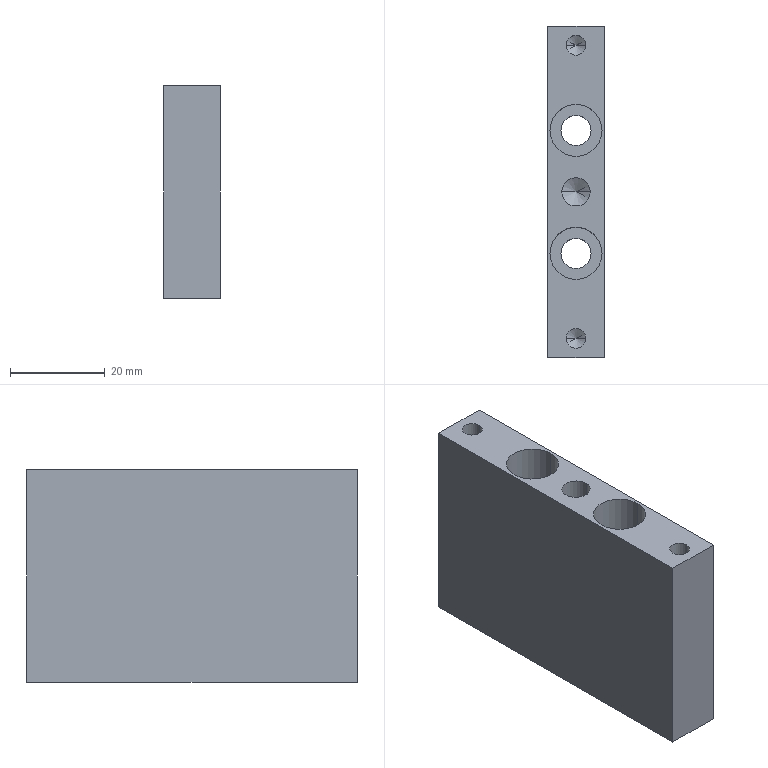Part | SolidWorks | features HoleWzd 5, Extrusion 1, MirrorPattern 1 | 1 solid | 42 faces | box 12 x 70 x 45 mm | volume 30841 mm3 | cylinder 22 | cone 12 | plane 8 | commonest cylinder face diameters 6 x6 2.5 x4 4.2 x4 6.4 x4 11 x4
STEP:
#1=CARTESIAN_POINT('',(3.,-22.5,10.));
#2=VERTEX_POINT('',#1);
#3=CARTESIAN_POINT('',(-3.,-22.5,10.));
#4=VERTEX_POINT('',#3);
#5=CARTESIAN_POINT('',(0.,-22.5,10.));
#6=DIRECTION('',(0.,0.,-1.));
#7=DIRECTION('',(-1.,0.,0.));
#8=AXIS2_PLACEMENT_3D('',#5,#6,#7);
#9=CIRCLE('',#8,3.);
#10=EDGE_CURVE('',#2,#4,#9,.T.);
#11=ORIENTED_EDGE('',*,*,#10,.F.);
#12=CARTESIAN_POINT('',(3.,-22.5,0.));
#13=VERTEX_POINT('',#12);
#14=CARTESIAN_POINT('',(3.,-22.5,0.));
#15=DIRECTION('',(0.,0.,-1.));
#16=VECTOR('',#15,1000.);
#17=LINE('',#14,#16);
#18=EDGE_CURVE('',#2,#13,#17,.T.);
#19=ORIENTED_EDGE('',*,*,#18,.T.);
#20=CARTESIAN_POINT('',(-3.,-22.5,0.));
#21=VERTEX_POINT('',#20);
#22=CARTESIAN_POINT('',(0.,-22.5,0.));
#23=DIRECTION('',(0.,0.,-1.));
#24=DIRECTION('',(-1.,0.,0.));
#25=AXIS2_PLACEMENT_3D('',#22,#23,#24);
#26=CIRCLE('',#25,3.);
#27=EDGE_CURVE('',#13,#21,#26,.T.);
#28=ORIENTED_EDGE('',*,*,#27,.T.);
#29=CARTESIAN_POINT('',(-3.,-22.5,0.));
#30=DIRECTION('',(0.,0.,-1.));
#31=VECTOR('',#30,1000.);
#32=LINE('',#29,#31);
#33=EDGE_CURVE('',#4,#21,#32,.T.);
#34=ORIENTED_EDGE('',*,*,#33,.F.);
#35=EDGE_LOOP('',(#11,#19,#28,#34));
#36=FACE_OUTER_BOUND('',#35,.T.);
#37=CARTESIAN_POINT('',(0.,-22.5,0.));
#38=DIRECTION('',(0.,0.,-1.));
#39=DIRECTION('',(-1.,0.,0.));
#40=AXIS2_PLACEMENT_3D('',#37,#38,#39);
#41=CYLINDRICAL_SURFACE('',#40,3.);
#42=ADVANCED_FACE('',(#36),#41,.F.);
#43=CARTESIAN_POINT('',(0.,-22.5,11.803));
#44=VERTEX_POINT('',#43);
#45=CARTESIAN_POINT('',(-3.,-22.5,10.));
#46=DIRECTION('',(-0.8572,0.,-0.515));
#47=VECTOR('',#46,1000.);
#48=LINE('',#45,#47);
#49=EDGE_CURVE('',#44,#4,#48,.T.);
#50=ORIENTED_EDGE('',*,*,#49,.F.);
#51=CARTESIAN_POINT('',(3.,-22.5,10.));
#52=DIRECTION('',(0.8572,0.,-0.515));
#53=VECTOR('',#52,1000.);
#54=LINE('',#51,#53);
#55=EDGE_CURVE('',#44,#2,#54,.T.);
#56=ORIENTED_EDGE('',*,*,#55,.T.);
#57=ORIENTED_EDGE('',*,*,#10,.T.);
#58=EDGE_LOOP('',(#50,#56,#57));
#59=FACE_OUTER_BOUND('',#58,.T.);
#60=CARTESIAN_POINT('',(0.,-22.5,10.));
#61=DIRECTION('',(0.,0.,-1.));
#62=DIRECTION('',(-1.,0.,0.));
#63=AXIS2_PLACEMENT_3D('',#60,#61,#62);
#64=CONICAL_SURFACE('',#63,3.,1.03);
#65=ADVANCED_FACE('',(#59),#64,.F.);
#66=CARTESIAN_POINT('',(0.,22.5,11.803));
#67=VERTEX_POINT('',#66);
#68=CARTESIAN_POINT('',(-3.,22.5,10.));
#69=VERTEX_POINT('',#68);
#70=CARTESIAN_POINT('',(-3.,22.5,10.));
#71=DIRECTION('',(-0.8572,0.,-0.515));
#72=VECTOR('',#71,1000.);
#73=LINE('',#70,#72);
#74=EDGE_CURVE('',#67,#69,#73,.T.);
#75=ORIENTED_EDGE('',*,*,#74,.F.);
#76=CARTESIAN_POINT('',(3.,22.5,10.));
#77=VERTEX_POINT('',#76);
#78=CARTESIAN_POINT('',(3.,22.5,10.));
#79=DIRECTION('',(0.8572,0.,-0.515));
#80=VECTOR('',#79,1000.);
#81=LINE('',#78,#80);
#82=EDGE_CURVE('',#67,#77,#81,.T.);
#83=ORIENTED_EDGE('',*,*,#82,.T.);
#84=CARTESIAN_POINT('',(0.,22.5,10.));
#85=DIRECTION('',(0.,0.,-1.));
#86=DIRECTION('',(-1.,0.,0.));
#87=AXIS2_PLACEMENT_3D('',#84,#85,#86);
#88=CIRCLE('',#87,3.);
#89=EDGE_CURVE('',#77,#69,#88,.T.);
#90=ORIENTED_EDGE('',*,*,#89,.T.);
#91=EDGE_LOOP('',(#75,#83,#90));
#92=FACE_OUTER_BOUND('',#91,.T.);
#93=CARTESIAN_POINT('',(0.,22.5,10.));
#94=DIRECTION('',(0.,0.,-1.));
#95=DIRECTION('',(-1.,0.,0.));
#96=AXIS2_PLACEMENT_3D('',#93,#94,#95);
#97=CONICAL_SURFACE('',#96,3.,1.03);
#98=ADVANCED_FACE('',(#92),#97,.F.);
#99=ORIENTED_EDGE('',*,*,#89,.F.);
#100=CARTESIAN_POINT('',(3.,22.5,0.));
#101=VERTEX_POINT('',#100);
#102=CARTESIAN_POINT('',(3.,22.5,0.));
#103=DIRECTION('',(0.,0.,-1.));
#104=VECTOR('',#103,1000.);
#105=LINE('',#102,#104);
#106=EDGE_CURVE('',#77,#101,#105,.T.);
#107=ORIENTED_EDGE('',*,*,#106,.T.);
#108=CARTESIAN_POINT('',(-3.,22.5,0.));
#109=VERTEX_POINT('',#108);
#110=CARTESIAN_POINT('',(0.,22.5,0.));
#111=DIRECTION('',(0.,0.,-1.));
#112=DIRECTION('',(-1.,0.,0.));
#113=AXIS2_PLACEMENT_3D('',#110,#111,#112);
#114=CIRCLE('',#113,3.);
#115=EDGE_CURVE('',#101,#109,#114,.T.);
#116=ORIENTED_EDGE('',*,*,#115,.T.);
#117=CARTESIAN_POINT('',(-3.,22.5,0.));
#118=DIRECTION('',(0.,0.,-1.));
#119=VECTOR('',#118,1000.);
#120=LINE('',#117,#119);
#121=EDGE_CURVE('',#69,#109,#120,.T.);
#122=ORIENTED_EDGE('',*,*,#121,.F.);
#123=EDGE_LOOP('',(#99,#107,#116,#122));
#124=FACE_OUTER_BOUND('',#123,.T.);
#125=CARTESIAN_POINT('',(0.,22.5,0.));
#126=DIRECTION('',(0.,0.,-1.));
#127=DIRECTION('',(-1.,0.,0.));
#128=AXIS2_PLACEMENT_3D('',#125,#126,#127);
#129=CYLINDRICAL_SURFACE('',#128,3.);
#130=ADVANCED_FACE('',(#124),#129,.F.);
#131=CARTESIAN_POINT('',(-3.,0.,35.));
#132=VERTEX_POINT('',#131);
#133=CARTESIAN_POINT('',(3.,0.,35.));
#134=VERTEX_POINT('',#133);
#135=CARTESIAN_POINT('',(0.,0.,35.));
#136=DIRECTION('',(0.,0.,1.));
#137=DIRECTION('',(1.,0.,0.));
#138=AXIS2_PLACEMENT_3D('',#135,#136,#137);
#139=CIRCLE('',#138,3.);
#140=EDGE_CURVE('',#132,#134,#139,.T.);
#141=ORIENTED_EDGE('',*,*,#140,.F.);
#142=CARTESIAN_POINT('',(-3.,0.,45.));
#143=VERTEX_POINT('',#142);
#144=CARTESIAN_POINT('',(-3.,0.,45.));
#145=DIRECTION('',(0.,0.,1.));
#146=VECTOR('',#145,1000.);
#147=LINE('',#144,#146);
#148=EDGE_CURVE('',#132,#143,#147,.T.);
#149=ORIENTED_EDGE('',*,*,#148,.T.);
#150=CARTESIAN_POINT('',(3.,0.,45.));
#151=VERTEX_POINT('',#150);
#152=CARTESIAN_POINT('',(0.,0.,45.));
#153=DIRECTION('',(0.,0.,1.));
#154=DIRECTION('',(1.,0.,0.));
#155=AXIS2_PLACEMENT_3D('',#152,#153,#154);
#156=CIRCLE('',#155,3.);
#157=EDGE_CURVE('',#143,#151,#156,.T.);
#158=ORIENTED_EDGE('',*,*,#157,.T.);
#159=CARTESIAN_POINT('',(3.,0.,45.));
#160=DIRECTION('',(0.,0.,1.));
#161=VECTOR('',#160,1000.);
#162=LINE('',#159,#161);
#163=EDGE_CURVE('',#134,#151,#162,.T.);
#164=ORIENTED_EDGE('',*,*,#163,.F.);
#165=EDGE_LOOP('',(#141,#149,#158,#164));
#166=FACE_OUTER_BOUND('',#165,.T.);
#167=CARTESIAN_POINT('',(0.,0.,45.));
#168=DIRECTION('',(0.,0.,1.));
#169=DIRECTION('',(1.,0.,0.));
#170=AXIS2_PLACEMENT_3D('',#167,#168,#169);
#171=CYLINDRICAL_SURFACE('',#170,3.);
#172=ADVANCED_FACE('',(#166),#171,.F.);
#173=CARTESIAN_POINT('',(0.,0.,33.197));
#174=VERTEX_POINT('',#173);
#175=CARTESIAN_POINT('',(3.,0.,35.));
#176=DIRECTION('',(0.8572,0.,0.515));
#177=VECTOR('',#176,1000.);
#178=LINE('',#175,#177);
#179=EDGE_CURVE('',#174,#134,#178,.T.);
#180=ORIENTED_EDGE('',*,*,#179,.F.);
#181=CARTESIAN_POINT('',(-3.,0.,35.));
#182=DIRECTION('',(-0.8572,0.,0.515));
#183=VECTOR('',#182,1000.);
#184=LINE('',#181,#183);
#185=EDGE_CURVE('',#174,#132,#184,.T.);
#186=ORIENTED_EDGE('',*,*,#185,.T.);
#187=ORIENTED_EDGE('',*,*,#140,.T.);
#188=EDGE_LOOP('',(#180,#186,#187));
#189=FACE_OUTER_BOUND('',#188,.T.);
#190=CARTESIAN_POINT('',(0.,0.,35.));
#191=DIRECTION('',(0.,0.,1.));
#192=DIRECTION('',(1.,0.,0.));
#193=AXIS2_PLACEMENT_3D('',#190,#191,#192);
#194=CONICAL_SURFACE('',#193,3.,1.03);
#195=ADVANCED_FACE('',(#189),#194,.F.);
#196=CARTESIAN_POINT('',(-5.5,13.,25.));
#197=VERTEX_POINT('',#196);
#198=CARTESIAN_POINT('',(5.5,13.,25.));
#199=VERTEX_POINT('',#198);
#200=CARTESIAN_POINT('',(0.,13.,25.));
#201=DIRECTION('',(0.,0.,1.));
#202=DIRECTION('',(1.,0.,0.));
#203=AXIS2_PLACEMENT_3D('',#200,#201,#202);
#204=CIRCLE('',#203,5.5);
#205=EDGE_CURVE('',#197,#199,#204,.T.);
#206=ORIENTED_EDGE('',*,*,#205,.F.);
#207=CARTESIAN_POINT('',(-5.5,13.,45.));
#208=VERTEX_POINT('',#207);
#209=CARTESIAN_POINT('',(-5.5,13.,45.));
#210=DIRECTION('',(0.,0.,1.));
#211=VECTOR('',#210,1000.);
#212=LINE('',#209,#211);
#213=EDGE_CURVE('',#197,#208,#212,.T.);
#214=ORIENTED_EDGE('',*,*,#213,.T.);
#215=CARTESIAN_POINT('',(5.5,13.,45.));
#216=VERTEX_POINT('',#215);
#217=CARTESIAN_POINT('',(0.,13.,45.));
#218=DIRECTION('',(0.,0.,1.));
#219=DIRECTION('',(1.,0.,0.));
#220=AXIS2_PLACEMENT_3D('',#217,#218,#219);
#221=CIRCLE('',#220,5.5);
#222=EDGE_CURVE('',#208,#216,#221,.T.);
#223=ORIENTED_EDGE('',*,*,#222,.T.);
#224=CARTESIAN_POINT('',(5.5,13.,45.));
#225=DIRECTION('',(0.,0.,1.));
#226=VECTOR('',#225,1000.);
#227=LINE('',#224,#226);
#228=EDGE_CURVE('',#199,#216,#227,.T.);
#229=ORIENTED_EDGE('',*,*,#228,.F.);
#230=EDGE_LOOP('',(#206,#214,#223,#229));
#231=FACE_OUTER_BOUND('',#230,.T.);
#232=CARTESIAN_POINT('',(0.,13.,45.));
#233=DIRECTION('',(0.,0.,1.));
#234=DIRECTION('',(1.,0.,0.));
#235=AXIS2_PLACEMENT_3D('',#232,#233,#234);
#236=CYLINDRICAL_SURFACE('',#235,5.5);
#237=ADVANCED_FACE('',(#231),#236,.F.);
#238=CARTESIAN_POINT('',(-3.2,13.,0.));
#239=VERTEX_POINT('',#238);
#240=CARTESIAN_POINT('',(3.2,13.,0.));
#241=VERTEX_POINT('',#240);
#242=CARTESIAN_POINT('',(0.,13.,0.));
#243=DIRECTION('',(0.,0.,1.));
#244=DIRECTION('',(1.,0.,0.));
#245=AXIS2_PLACEMENT_3D('',#242,#243,#244);
#246=CIRCLE('',#245,3.2);
#247=EDGE_CURVE('',#239,#241,#246,.T.);
#248=ORIENTED_EDGE('',*,*,#247,.F.);
#249=CARTESIAN_POINT('',(-3.2,13.,25.));
#250=VERTEX_POINT('',#249);
#251=CARTESIAN_POINT('',(-3.2,13.,45.));
#252=DIRECTION('',(0.,0.,1.));
#253=VECTOR('',#252,1000.);
#254=LINE('',#251,#253);
#255=EDGE_CURVE('',#239,#250,#254,.T.);
#256=ORIENTED_EDGE('',*,*,#255,.T.);
#257=CARTESIAN_POINT('',(3.2,13.,25.));
#258=VERTEX_POINT('',#257);
#259=CARTESIAN_POINT('',(0.,13.,25.));
#260=DIRECTION('',(0.,0.,1.));
#261=DIRECTION('',(1.,0.,0.));
#262=AXIS2_PLACEMENT_3D('',#259,#260,#261);
#263=CIRCLE('',#262,3.2);
#264=EDGE_CURVE('',#250,#258,#263,.T.);
#265=ORIENTED_EDGE('',*,*,#264,.T.);
#266=CARTESIAN_POINT('',(3.2,13.,45.));
#267=DIRECTION('',(0.,0.,1.));
#268=VECTOR('',#267,1000.);
#269=LINE('',#266,#268);
#270=EDGE_CURVE('',#241,#258,#269,.T.);
#271=ORIENTED_EDGE('',*,*,#270,.F.);
#272=EDGE_LOOP('',(#248,#256,#265,#271));
#273=FACE_OUTER_BOUND('',#272,.T.);
#274=CARTESIAN_POINT('',(0.,13.,45.));
#275=DIRECTION('',(0.,0.,1.));
#276=DIRECTION('',(1.,0.,0.));
#277=AXIS2_PLACEMENT_3D('',#274,#275,#276);
#278=CYLINDRICAL_SURFACE('',#277,3.2);
#279=ADVANCED_FACE('',(#273),#278,.F.);
#280=CARTESIAN_POINT('',(-5.5,-13.,25.));
#281=VERTEX_POINT('',#280);
#282=CARTESIAN_POINT('',(5.5,-13.,25.));
#283=VERTEX_POINT('',#282);
#284=CARTESIAN_POINT('',(0.,-13.,25.));
#285=DIRECTION('',(0.,0.,1.));
#286=DIRECTION('',(1.,0.,0.));
#287=AXIS2_PLACEMENT_3D('',#284,#285,#286);
#288=CIRCLE('',#287,5.5);
#289=EDGE_CURVE('',#281,#283,#288,.T.);
#290=ORIENTED_EDGE('',*,*,#289,.F.);
#291=CARTESIAN_POINT('',(-5.5,-13.,45.));
#292=VERTEX_POINT('',#291);
#293=CARTESIAN_POINT('',(-5.5,-13.,45.));
#294=DIRECTION('',(0.,0.,1.));
#295=VECTOR('',#294,1000.);
#296=LINE('',#293,#295);
#297=EDGE_CURVE('',#281,#292,#296,.T.);
#298=ORIENTED_EDGE('',*,*,#297,.T.);
#299=CARTESIAN_POINT('',(5.5,-13.,45.));
#300=VERTEX_POINT('',#299);
#301=CARTESIAN_POINT('',(0.,-13.,45.));
#302=DIRECTION('',(0.,0.,1.));
#303=DIRECTION('',(1.,0.,0.));
#304=AXIS2_PLACEMENT_3D('',#301,#302,#303);
#305=CIRCLE('',#304,5.5);
#306=EDGE_CURVE('',#292,#300,#305,.T.);
#307=ORIENTED_EDGE('',*,*,#306,.T.);
#308=CARTESIAN_POINT('',(5.5,-13.,45.));
#309=DIRECTION('',(0.,0.,1.));
#310=VECTOR('',#309,1000.);
#311=LINE('',#308,#310);
#312=EDGE_CURVE('',#283,#300,#311,.T.);
#313=ORIENTED_EDGE('',*,*,#312,.F.);
#314=EDGE_LOOP('',(#290,#298,#307,#313));
#315=FACE_OUTER_BOUND('',#314,.T.);
#316=CARTESIAN_POINT('',(0.,-13.,45.));
#317=DIRECTION('',(0.,0.,1.));
#318=DIRECTION('',(1.,0.,0.));
#319=AXIS2_PLACEMENT_3D('',#316,#317,#318);
#320=CYLINDRICAL_SURFACE('',#319,5.5);
#321=ADVANCED_FACE('',(#315),#320,.F.);
#322=CARTESIAN_POINT('',(-3.2,-13.,0.));
#323=VERTEX_POINT('',#322);
#324=CARTESIAN_POINT('',(3.2,-13.,0.));
#325=VERTEX_POINT('',#324);
#326=CARTESIAN_POINT('',(0.,-13.,0.));
#327=DIRECTION('',(0.,0.,1.));
#328=DIRECTION('',(1.,0.,0.));
#329=AXIS2_PLACEMENT_3D('',#326,#327,#328);
#330=CIRCLE('',#329,3.2);
#331=EDGE_CURVE('',#323,#325,#330,.T.);
#332=ORIENTED_EDGE('',*,*,#331,.F.);
#333=CARTESIAN_POINT('',(-3.2,-13.,25.));
#334=VERTEX_POINT('',#333);
#335=CARTESIAN_POINT('',(-3.2,-13.,45.));
#336=DIRECTION('',(0.,0.,1.));
#337=VECTOR('',#336,1000.);
#338=LINE('',#335,#337);
#339=EDGE_CURVE('',#323,#334,#338,.T.);
#340=ORIENTED_EDGE('',*,*,#339,.T.);
#341=CARTESIAN_POINT('',(3.2,-13.,25.));
#342=VERTEX_POINT('',#341);
#343=CARTESIAN_POINT('',(0.,-13.,25.));
#344=DIRECTION('',(0.,0.,1.));
#345=DIRECTION('',(1.,0.,0.));
#346=AXIS2_PLACEMENT_3D('',#343,#344,#345);
#347=CIRCLE('',#346,3.2);
#348=EDGE_CURVE('',#334,#342,#347,.T.);
#349=ORIENTED_EDGE('',*,*,#348,.T.);
#350=CARTESIAN_POINT('',(3.2,-13.,45.));
#351=DIRECTION('',(0.,0.,1.));
#352=VECTOR('',#351,1000.);
#353=LINE('',#350,#352);
#354=EDGE_CURVE('',#325,#342,#353,.T.);
#355=ORIENTED_EDGE('',*,*,#354,.F.);
#356=EDGE_LOOP('',(#332,#340,#349,#355));
#357=FACE_OUTER_BOUND('',#356,.T.);
#358=CARTESIAN_POINT('',(0.,-13.,45.));
#359=DIRECTION('',(0.,0.,1.));
#360=DIRECTION('',(1.,0.,0.));
#361=AXIS2_PLACEMENT_3D('',#358,#359,#360);
#362=CYLINDRICAL_SURFACE('',#361,3.2);
#363=ADVANCED_FACE('',(#357),#362,.F.);
#364=CARTESIAN_POINT('',(-2.1,31.,26.));
#365=VERTEX_POINT('',#364);
#366=CARTESIAN_POINT('',(2.1,31.,26.));
#367=VERTEX_POINT('',#366);
#368=CARTESIAN_POINT('',(0.,31.,26.));
#369=DIRECTION('',(0.,0.,1.));
#370=DIRECTION('',(1.,0.,0.));
#371=AXIS2_PLACEMENT_3D('',#368,#369,#370);
#372=CIRCLE('',#371,2.1);
#373=EDGE_CURVE('',#365,#367,#372,.T.);
#374=ORIENTED_EDGE('',*,*,#373,.F.);
#375=CARTESIAN_POINT('',(-2.1,31.,45.));
#376=VERTEX_POINT('',#375);
#377=CARTESIAN_POINT('',(-2.1,31.,45.));
#378=DIRECTION('',(0.,0.,1.));
#379=VECTOR('',#378,1000.);
#380=LINE('',#377,#379);
#381=EDGE_CURVE('',#365,#376,#380,.T.);
#382=ORIENTED_EDGE('',*,*,#381,.T.);
#383=CARTESIAN_POINT('',(2.1,31.,45.));
#384=VERTEX_POINT('',#383);
#385=CARTESIAN_POINT('',(0.,31.,45.));
#386=DIRECTION('',(0.,0.,1.));
#387=DIRECTION('',(1.,0.,0.));
#388=AXIS2_PLACEMENT_3D('',#385,#386,#387);
#389=CIRCLE('',#388,2.1);
#390=EDGE_CURVE('',#376,#384,#389,.T.);
#391=ORIENTED_EDGE('',*,*,#390,.T.);
#392=CARTESIAN_POINT('',(2.1,31.,45.));
#393=DIRECTION('',(0.,0.,1.));
#394=VECTOR('',#393,1000.);
#395=LINE('',#392,#394);
#396=EDGE_CURVE('',#367,#384,#395,.T.);
#397=ORIENTED_EDGE('',*,*,#396,.F.);
#398=EDGE_LOOP('',(#374,#382,#391,#397));
#399=FACE_OUTER_BOUND('',#398,.T.);
#400=CARTESIAN_POINT('',(0.,31.,45.));
#401=DIRECTION('',(0.,0.,1.));
#402=DIRECTION('',(1.,0.,0.));
#403=AXIS2_PLACEMENT_3D('',#400,#401,#402);
#404=CYLINDRICAL_SURFACE('',#403,2.1);
#405=ADVANCED_FACE('',(#399),#404,.F.);
#406=CARTESIAN_POINT('',(0.,31.,24.738));
#407=VERTEX_POINT('',#406);
#408=CARTESIAN_POINT('',(2.1,31.,26.));
#409=DIRECTION('',(0.8572,0.,0.515));
#410=VECTOR('',#409,1000.);
#411=LINE('',#408,#410);
#412=EDGE_CURVE('',#407,#367,#411,.T.);
#413=ORIENTED_EDGE('',*,*,#412,.F.);
#414=CARTESIAN_POINT('',(-2.1,31.,26.));
#415=DIRECTION('',(-0.8572,0.,0.515));
#416=VECTOR('',#415,1000.);
#417=LINE('',#414,#416);
#418=EDGE_CURVE('',#407,#365,#417,.T.);
#419=ORIENTED_EDGE('',*,*,#418,.T.);
#420=ORIENTED_EDGE('',*,*,#373,.T.);
#421=EDGE_LOOP('',(#413,#419,#420));
#422=FACE_OUTER_BOUND('',#421,.T.);
#423=CARTESIAN_POINT('',(0.,31.,26.));
#424=DIRECTION('',(0.,0.,1.));
#425=DIRECTION('',(1.,0.,0.));
#426=AXIS2_PLACEMENT_3D('',#423,#424,#425);
#427=CONICAL_SURFACE('',#426,2.1,1.03);
#428=ADVANCED_FACE('',(#422),#427,.F.);
#429=CARTESIAN_POINT('',(-2.1,-31.,26.));
#430=VERTEX_POINT('',#429);
#431=CARTESIAN_POINT('',(2.1,-31.,26.));
#432=VERTEX_POINT('',#431);
#433=CARTESIAN_POINT('',(0.,-31.,26.));
#434=DIRECTION('',(0.,0.,1.));
#435=DIRECTION('',(1.,0.,0.));
#436=AXIS2_PLACEMENT_3D('',#433,#434,#435);
#437=CIRCLE('',#436,2.1);
#438=EDGE_CURVE('',#430,#432,#437,.T.);
#439=ORIENTED_EDGE('',*,*,#438,.F.);
#440=CARTESIAN_POINT('',(-2.1,-31.,45.));
#441=VERTEX_POINT('',#440);
#442=CARTESIAN_POINT('',(-2.1,-31.,45.));
#443=DIRECTION('',(0.,0.,1.));
#444=VECTOR('',#443,1000.);
#445=LINE('',#442,#444);
#446=EDGE_CURVE('',#430,#441,#445,.T.);
#447=ORIENTED_EDGE('',*,*,#446,.T.);
#448=CARTESIAN_POINT('',(2.1,-31.,45.));
#449=VERTEX_POINT('',#448);
#450=CARTESIAN_POINT('',(0.,-31.,45.));
#451=DIRECTION('',(0.,0.,1.));
#452=DIRECTION('',(1.,0.,0.));
#453=AXIS2_PLACEMENT_3D('',#450,#451,#452);
#454=CIRCLE('',#453,2.1);
#455=EDGE_CURVE('',#441,#449,#454,.T.);
#456=ORIENTED_EDGE('',*,*,#455,.T.);
#457=CARTESIAN_POINT('',(2.1,-31.,45.));
#458=DIRECTION('',(0.,0.,1.));
#459=VECTOR('',#458,1000.);
#460=LINE('',#457,#459);
#461=EDGE_CURVE('',#432,#449,#460,.T.);
#462=ORIENTED_EDGE('',*,*,#461,.F.);
#463=EDGE_LOOP('',(#439,#447,#456,#462));
#464=FACE_OUTER_BOUND('',#463,.T.);
#465=CARTESIAN_POINT('',(0.,-31.,45.));
#466=DIRECTION('',(0.,0.,1.));
#467=DIRECTION('',(1.,0.,0.));
#468=AXIS2_PLACEMENT_3D('',#465,#466,#467);
#469=CYLINDRICAL_SURFACE('',#468,2.1);
#470=ADVANCED_FACE('',(#464),#469,.F.);
#471=CARTESIAN_POINT('',(0.,-31.,24.738));
#472=VERTEX_POINT('',#471);
#473=CARTESIAN_POINT('',(2.1,-31.,26.));
#474=DIRECTION('',(0.8572,0.,0.515));
#475=VECTOR('',#474,1000.);
#476=LINE('',#473,#475);
#477=EDGE_CURVE('',#472,#432,#476,.T.);
#478=ORIENTED_EDGE('',*,*,#477,.F.);
#479=CARTESIAN_POINT('',(-2.1,-31.,26.));
#480=DIRECTION('',(-0.8572,0.,0.515));
#481=VECTOR('',#480,1000.);
#482=LINE('',#479,#481);
#483=EDGE_CURVE('',#472,#430,#482,.T.);
#484=ORIENTED_EDGE('',*,*,#483,.T.);
#485=ORIENTED_EDGE('',*,*,#438,.T.);
#486=EDGE_LOOP('',(#478,#484,#485));
#487=FACE_OUTER_BOUND('',#486,.T.);
#488=CARTESIAN_POINT('',(0.,-31.,26.));
#489=DIRECTION('',(0.,0.,1.));
#490=DIRECTION('',(1.,0.,0.));
#491=AXIS2_PLACEMENT_3D('',#488,#489,#490);
#492=CONICAL_SURFACE('',#491,2.1,1.03);
#493=ADVANCED_FACE('',(#487),#492,.F.);
#494=CARTESIAN_POINT('',(-1.25,25.227,10.));
#495=VERTEX_POINT('',#494);
#496=CARTESIAN_POINT('',(0.,25.5,8.75));
#497=VERTEX_POINT('',#496);
#498=CARTESIAN_POINT('',(-1.25,25.227,10.));
#499=CARTESIAN_POINT('',(-1.25,25.227,9.916));
#500=CARTESIAN_POINT('',(-1.242,25.231,9.834));
#501=CARTESIAN_POINT('',(-1.209,25.246,9.673));
#502=CARTESIAN_POINT('',(-1.185,25.256,9.593));
#503=CARTESIAN_POINT('',(-1.09,25.296,9.367));
#504=CARTESIAN_POINT('',(-0.9976,25.332,9.23));
#505=CARTESIAN_POINT('',(-0.7697,25.402,9.002));
#506=CARTESIAN_POINT('',(-0.6318,25.437,8.909));
#507=CARTESIAN_POINT('',(-0.3312,25.486,8.784));
#508=CARTESIAN_POINT('',(-0.1654,25.5,8.75));
#509=CARTESIAN_POINT('',(0.,25.5,8.75));
#510=B_SPLINE_CURVE_WITH_KNOTS('',3,(#498,#499,#500,#501,#502,#503,#504,#505,#506,#507,#508,#509),.UNSPECIFIED.,.F.,.F.,(4,2,2,2,2,4),(0.,0.0002472,0.0004943,0.0009887,0.001483,0.001977),.UNSPECIFIED.);
#511=EDGE_CURVE('',#495,#497,#510,.T.);
#512=ORIENTED_EDGE('',*,*,#511,.T.);
#513=CARTESIAN_POINT('',(0.,35.,8.75));
#514=VERTEX_POINT('',#513);
#515=CARTESIAN_POINT('',(0.,35.,8.75));
#516=DIRECTION('',(0.,1.,0.));
#517=VECTOR('',#516,1000.);
#518=LINE('',#515,#517);
#519=EDGE_CURVE('',#497,#514,#518,.T.);
#520=ORIENTED_EDGE('',*,*,#519,.T.);
#521=CARTESIAN_POINT('',(0.,35.,11.25));
#522=VERTEX_POINT('',#521);
#523=CARTESIAN_POINT('',(0.,35.,10.));
#524=DIRECTION('',(0.,1.,0.));
#525=DIRECTION('',(0.,0.,1.));
#526=AXIS2_PLACEMENT_3D('',#523,#524,#525);
#527=CIRCLE('',#526,1.25);
#528=EDGE_CURVE('',#514,#522,#527,.T.);
#529=ORIENTED_EDGE('',*,*,#528,.T.);
#530=CARTESIAN_POINT('',(0.,23.42,11.25));
#531=VERTEX_POINT('',#530);
#532=CARTESIAN_POINT('',(0.,35.,11.25));
#533=DIRECTION('',(0.,1.,0.));
#534=VECTOR('',#533,1000.);
#535=LINE('',#532,#534);
#536=EDGE_CURVE('',#531,#522,#535,.T.);
#537=ORIENTED_EDGE('',*,*,#536,.F.);
#538=CARTESIAN_POINT('',(0.,23.42,11.25));
#539=CARTESIAN_POINT('',(-0.1196,23.42,11.25));
#540=CARTESIAN_POINT('',(-0.2373,23.423,11.233));
#541=CARTESIAN_POINT('',(-0.4653,23.457,11.166));
#542=CARTESIAN_POINT('',(-0.5713,23.489,11.117));
#543=CARTESIAN_POINT('',(-0.7516,23.596,11.004));
#544=CARTESIAN_POINT('',(-0.8259,23.67,10.942));
#545=CARTESIAN_POINT('',(-0.9473,23.833,10.82));
#546=CARTESIAN_POINT('',(-0.9958,23.923,10.759));
#547=CARTESIAN_POINT('',(-1.118,24.205,10.577));
#548=CARTESIAN_POINT('',(-1.168,24.404,10.461));
#549=CARTESIAN_POINT('',(-1.235,24.811,10.229));
#550=CARTESIAN_POINT('',(-1.25,25.019,10.114));
#551=CARTESIAN_POINT('',(-1.25,25.227,10.));
#552=B_SPLINE_CURVE_WITH_KNOTS('',3,(#538,#539,#540,#541,#542,#543,#544,#545,#546,#547,#548,#549,#550,#551),.UNSPECIFIED.,.F.,.F.,(4,2,2,2,2,2,4),(0.003073,0.003423,0.003774,0.004124,0.004474,0.005175,0.005875),.UNSPECIFIED.);
#553=EDGE_CURVE('',#531,#495,#552,.T.);
#554=ORIENTED_EDGE('',*,*,#553,.T.);
#555=EDGE_LOOP('',(#512,#520,#529,#537,#554));
#556=FACE_OUTER_BOUND('',#555,.T.);
#557=CARTESIAN_POINT('',(0.,35.,10.));
#558=DIRECTION('',(0.,1.,0.));
#559=DIRECTION('',(0.,0.,1.));
#560=AXIS2_PLACEMENT_3D('',#557,#558,#559);
#561=CYLINDRICAL_SURFACE('',#560,1.25);
#562=ADVANCED_FACE('',(#556),#561,.F.);
#563=CARTESIAN_POINT('',(0.,22.5,14.75));
#564=VERTEX_POINT('',#563);
#565=CARTESIAN_POINT('',(0.,22.5,17.25));
#566=VERTEX_POINT('',#565);
#567=CARTESIAN_POINT('',(0.,22.5,16.));
#568=DIRECTION('',(0.,1.,0.));
#569=DIRECTION('',(0.,0.,1.));
#570=AXIS2_PLACEMENT_3D('',#567,#568,#569);
#571=CIRCLE('',#570,1.25);
#572=EDGE_CURVE('',#564,#566,#571,.T.);
#573=ORIENTED_EDGE('',*,*,#572,.F.);
#574=CARTESIAN_POINT('',(0.,35.,14.75));
#575=VERTEX_POINT('',#574);
#576=CARTESIAN_POINT('',(0.,35.,14.75));
#577=DIRECTION('',(0.,1.,0.));
#578=VECTOR('',#577,1000.);
#579=LINE('',#576,#578);
#580=EDGE_CURVE('',#564,#575,#579,.T.);
#581=ORIENTED_EDGE('',*,*,#580,.T.);
#582=CARTESIAN_POINT('',(0.,35.,17.25));
#583=VERTEX_POINT('',#582);
#584=CARTESIAN_POINT('',(0.,35.,16.));
#585=DIRECTION('',(0.,1.,0.));
#586=DIRECTION('',(0.,0.,1.));
#587=AXIS2_PLACEMENT_3D('',#584,#585,#586);
#588=CIRCLE('',#587,1.25);
#589=EDGE_CURVE('',#575,#583,#588,.T.);
#590=ORIENTED_EDGE('',*,*,#589,.T.);
#591=CARTESIAN_POINT('',(0.,35.,17.25));
#592=DIRECTION('',(0.,1.,0.));
#593=VECTOR('',#592,1000.);
#594=LINE('',#591,#593);
#595=EDGE_CURVE('',#566,#583,#594,.T.);
#596=ORIENTED_EDGE('',*,*,#595,.F.);
#597=EDGE_LOOP('',(#573,#581,#590,#596));
#598=FACE_OUTER_BOUND('',#597,.T.);
#599=CARTESIAN_POINT('',(0.,35.,16.));
#600=DIRECTION('',(0.,1.,0.));
#601=DIRECTION('',(0.,0.,1.));
#602=AXIS2_PLACEMENT_3D('',#599,#600,#601);
#603=CYLINDRICAL_SURFACE('',#602,1.25);
#604=ADVANCED_FACE('',(#598),#603,.F.);
#605=CARTESIAN_POINT('',(0.,21.749,16.));
#606=VERTEX_POINT('',#605);
#607=CARTESIAN_POINT('',(0.,22.5,17.25));
#608=DIRECTION('',(0.,0.515,0.8572));
#609=VECTOR('',#608,1000.);
#610=LINE('',#607,#609);
#611=EDGE_CURVE('',#606,#566,#610,.T.);
#612=ORIENTED_EDGE('',*,*,#611,.F.);
#613=CARTESIAN_POINT('',(0.,22.5,14.75));
#614=DIRECTION('',(0.,0.515,-0.8572));
#615=VECTOR('',#614,1000.);
#616=LINE('',#613,#615);
#617=EDGE_CURVE('',#606,#564,#616,.T.);
#618=ORIENTED_EDGE('',*,*,#617,.T.);
#619=ORIENTED_EDGE('',*,*,#572,.T.);
#620=EDGE_LOOP('',(#612,#618,#619));
#621=FACE_OUTER_BOUND('',#620,.T.);
#622=CARTESIAN_POINT('',(0.,22.5,16.));
#623=DIRECTION('',(0.,1.,0.));
#624=DIRECTION('',(0.,0.,1.));
#625=AXIS2_PLACEMENT_3D('',#622,#623,#624);
#626=CONICAL_SURFACE('',#625,1.25,1.03);
#627=ADVANCED_FACE('',(#621),#626,.F.);
#628=CARTESIAN_POINT('',(6.,-35.,0.));
#629=VERTEX_POINT('',#628);
#630=CARTESIAN_POINT('',(6.,35.,0.));
#631=VERTEX_POINT('',#630);
#632=CARTESIAN_POINT('',(6.,35.,0.));
#633=DIRECTION('',(0.,1.,0.));
#634=VECTOR('',#633,1000.);
#635=LINE('',#632,#634);
#636=EDGE_CURVE('',#629,#631,#635,.T.);
#637=ORIENTED_EDGE('',*,*,#636,.T.);
#638=CARTESIAN_POINT('',(6.,35.,45.));
#639=VERTEX_POINT('',#638);
#640=CARTESIAN_POINT('',(6.,35.,45.));
#641=DIRECTION('',(0.,0.,-1.));
#642=VECTOR('',#641,1000.);
#643=LINE('',#640,#642);
#644=EDGE_CURVE('',#639,#631,#643,.T.);
#645=ORIENTED_EDGE('',*,*,#644,.F.);
#646=CARTESIAN_POINT('',(6.,-35.,45.));
#647=VERTEX_POINT('',#646);
#648=CARTESIAN_POINT('',(6.,35.,45.));
#649=DIRECTION('',(0.,1.,0.));
#650=VECTOR('',#649,1000.);
#651=LINE('',#648,#650);
#652=EDGE_CURVE('',#647,#639,#651,.T.);
#653=ORIENTED_EDGE('',*,*,#652,.F.);
#654=CARTESIAN_POINT('',(6.,-35.,45.));
#655=DIRECTION('',(0.,0.,-1.));
#656=VECTOR('',#655,1000.);
#657=LINE('',#654,#656);
#658=EDGE_CURVE('',#647,#629,#657,.T.);
#659=ORIENTED_EDGE('',*,*,#658,.T.);
#660=EDGE_LOOP('',(#637,#645,#653,#659));
#661=FACE_OUTER_BOUND('',#660,.T.);
#662=CARTESIAN_POINT('',(6.,35.,45.));
#663=DIRECTION('',(-1.,0.,0.));
#664=DIRECTION('',(0.,-1.,0.));
#665=AXIS2_PLACEMENT_3D('',#662,#663,#664);
#666=PLANE('',#665);
#667=ADVANCED_FACE('',(#661),#666,.F.);
#668=CARTESIAN_POINT('',(0.,35.,10.));
#669=DIRECTION('',(0.,1.,0.));
#670=DIRECTION('',(0.,0.,1.));
#671=AXIS2_PLACEMENT_3D('',#668,#669,#670);
#672=CIRCLE('',#671,1.25);
#673=EDGE_CURVE('',#522,#514,#672,.T.);
#674=ORIENTED_EDGE('',*,*,#673,.F.);
#675=ORIENTED_EDGE('',*,*,#528,.F.);
#676=EDGE_LOOP('',(#674,#675));
#677=FACE_BOUND('',#676,.T.);
#678=CARTESIAN_POINT('',(0.,35.,16.));
#679=DIRECTION('',(0.,1.,0.));
#680=DIRECTION('',(0.,0.,1.));
#681=AXIS2_PLACEMENT_3D('',#678,#679,#680);
#682=CIRCLE('',#681,1.25);
#683=EDGE_CURVE('',#583,#575,#682,.T.);
#684=ORIENTED_EDGE('',*,*,#683,.F.);
#685=ORIENTED_EDGE('',*,*,#589,.F.);
#686=EDGE_LOOP('',(#684,#685));
#687=FACE_BOUND('',#686,.T.);
#688=CARTESIAN_POINT('',(-6.,35.,0.));
#689=VERTEX_POINT('',#688);
#690=CARTESIAN_POINT('',(-6.,35.,0.));
#691=DIRECTION('',(-1.,0.,0.));
#692=VECTOR('',#691,1000.);
#693=LINE('',#690,#692);
#694=EDGE_CURVE('',#631,#689,#693,.T.);
#695=ORIENTED_EDGE('',*,*,#694,.T.);
#696=CARTESIAN_POINT('',(-6.,35.,45.));
#697=VERTEX_POINT('',#696);
#698=CARTESIAN_POINT('',(-6.,35.,45.));
#699=DIRECTION('',(0.,0.,-1.));
#700=VECTOR('',#699,1000.);
#701=LINE('',#698,#700);
#702=EDGE_CURVE('',#697,#689,#701,.T.);
#703=ORIENTED_EDGE('',*,*,#702,.F.);
#704=CARTESIAN_POINT('',(-6.,35.,45.));
#705=DIRECTION('',(-1.,0.,0.));
#706=VECTOR('',#705,1000.);
#707=LINE('',#704,#706);
#708=EDGE_CURVE('',#639,#697,#707,.T.);
#709=ORIENTED_EDGE('',*,*,#708,.F.);
#710=ORIENTED_EDGE('',*,*,#644,.T.);
#711=EDGE_LOOP('',(#695,#703,#709,#710));
#712=FACE_OUTER_BOUND('',#711,.T.);
#713=CARTESIAN_POINT('',(-6.,35.,45.));
#714=DIRECTION('',(0.,-1.,0.));
#715=DIRECTION('',(0.,0.,-1.));
#716=AXIS2_PLACEMENT_3D('',#713,#714,#715);
#717=PLANE('',#716);
#718=ADVANCED_FACE('',(#677,#687,#712),#717,.F.);
#719=CARTESIAN_POINT('',(-6.,-35.,0.));
#720=VERTEX_POINT('',#719);
#721=CARTESIAN_POINT('',(-6.,35.,0.));
#722=DIRECTION('',(0.,-1.,0.));
#723=VECTOR('',#722,1000.);
#724=LINE('',#721,#723);
#725=EDGE_CURVE('',#689,#720,#724,.T.);
#726=ORIENTED_EDGE('',*,*,#725,.T.);
#727=CARTESIAN_POINT('',(-6.,-35.,45.));
#728=VERTEX_POINT('',#727);
#729=CARTESIAN_POINT('',(-6.,-35.,45.));
#730=DIRECTION('',(0.,0.,-1.));
#731=VECTOR('',#730,1000.);
#732=LINE('',#729,#731);
#733=EDGE_CURVE('',#728,#720,#732,.T.);
#734=ORIENTED_EDGE('',*,*,#733,.F.);
#735=CARTESIAN_POINT('',(-6.,35.,45.));
#736=DIRECTION('',(0.,-1.,0.));
#737=VECTOR('',#736,1000.);
#738=LINE('',#735,#737);
#739=EDGE_CURVE('',#697,#728,#738,.T.);
#740=ORIENTED_EDGE('',*,*,#739,.F.);
#741=ORIENTED_EDGE('',*,*,#702,.T.);
#742=EDGE_LOOP('',(#726,#734,#740,#741));
#743=FACE_OUTER_BOUND('',#742,.T.);
#744=CARTESIAN_POINT('',(-6.,35.,45.));
#745=DIRECTION('',(1.,0.,0.));
#746=DIRECTION('',(0.,1.,0.));
#747=AXIS2_PLACEMENT_3D('',#744,#745,#746);
#748=PLANE('',#747);
#749=ADVANCED_FACE('',(#743),#748,.F.);
#750=CARTESIAN_POINT('',(-6.,-35.,0.));
#751=DIRECTION('',(1.,0.,0.));
#752=VECTOR('',#751,1000.);
#753=LINE('',#750,#752);
#754=EDGE_CURVE('',#720,#629,#753,.T.);
#755=ORIENTED_EDGE('',*,*,#754,.T.);
#756=ORIENTED_EDGE('',*,*,#658,.F.);
#757=CARTESIAN_POINT('',(-6.,-35.,45.));
#758=DIRECTION('',(1.,0.,0.));
#759=VECTOR('',#758,1000.);
#760=LINE('',#757,#759);
#761=EDGE_CURVE('',#728,#647,#760,.T.);
#762=ORIENTED_EDGE('',*,*,#761,.F.);
#763=ORIENTED_EDGE('',*,*,#733,.T.);
#764=EDGE_LOOP('',(#755,#756,#762,#763));
#765=FACE_OUTER_BOUND('',#764,.T.);
#766=CARTESIAN_POINT('',(-6.,-35.,45.));
#767=DIRECTION('',(0.,1.,0.));
#768=DIRECTION('',(0.,0.,1.));
#769=AXIS2_PLACEMENT_3D('',#766,#767,#768);
#770=PLANE('',#769);
#771=ADVANCED_FACE('',(#765),#770,.F.);
#772=CARTESIAN_POINT('',(0.,0.,45.));
#773=DIRECTION('',(0.,0.,1.));
#774=DIRECTION('',(1.,0.,0.));
#775=AXIS2_PLACEMENT_3D('',#772,#773,#774);
#776=CIRCLE('',#775,3.);
#777=EDGE_CURVE('',#151,#143,#776,.T.);
#778=ORIENTED_EDGE('',*,*,#777,.F.);
#779=ORIENTED_EDGE('',*,*,#157,.F.);
#780=EDGE_LOOP('',(#778,#779));
#781=FACE_BOUND('',#780,.T.);
#782=CARTESIAN_POINT('',(0.,13.,45.));
#783=DIRECTION('',(0.,0.,1.));
#784=DIRECTION('',(1.,0.,0.));
#785=AXIS2_PLACEMENT_3D('',#782,#783,#784);
#786=CIRCLE('',#785,5.5);
#787=EDGE_CURVE('',#216,#208,#786,.T.);
#788=ORIENTED_EDGE('',*,*,#787,.F.);
#789=ORIENTED_EDGE('',*,*,#222,.F.);
#790=EDGE_LOOP('',(#788,#789));
#791=FACE_BOUND('',#790,.T.);
#792=CARTESIAN_POINT('',(0.,-13.,45.));
#793=DIRECTION('',(0.,0.,1.));
#794=DIRECTION('',(1.,0.,0.));
#795=AXIS2_PLACEMENT_3D('',#792,#793,#794);
#796=CIRCLE('',#795,5.5);
#797=EDGE_CURVE('',#300,#292,#796,.T.);
#798=ORIENTED_EDGE('',*,*,#797,.F.);
#799=ORIENTED_EDGE('',*,*,#306,.F.);
#800=EDGE_LOOP('',(#798,#799));
#801=FACE_BOUND('',#800,.T.);
#802=CARTESIAN_POINT('',(0.,31.,45.));
#803=DIRECTION('',(0.,0.,1.));
#804=DIRECTION('',(1.,0.,0.));
#805=AXIS2_PLACEMENT_3D('',#802,#803,#804);
#806=CIRCLE('',#805,2.1);
#807=EDGE_CURVE('',#384,#376,#806,.T.);
#808=ORIENTED_EDGE('',*,*,#807,.F.);
#809=ORIENTED_EDGE('',*,*,#390,.F.);
#810=EDGE_LOOP('',(#808,#809));
#811=FACE_BOUND('',#810,.T.);
#812=CARTESIAN_POINT('',(0.,-31.,45.));
#813=DIRECTION('',(0.,0.,1.));
#814=DIRECTION('',(1.,0.,0.));
#815=AXIS2_PLACEMENT_3D('',#812,#813,#814);
#816=CIRCLE('',#815,2.1);
#817=EDGE_CURVE('',#449,#441,#816,.T.);
#818=ORIENTED_EDGE('',*,*,#817,.F.);
#819=ORIENTED_EDGE('',*,*,#455,.F.);
#820=EDGE_LOOP('',(#818,#819));
#821=FACE_BOUND('',#820,.T.);
#822=ORIENTED_EDGE('',*,*,#652,.T.);
#823=ORIENTED_EDGE('',*,*,#708,.T.);
#824=ORIENTED_EDGE('',*,*,#739,.T.);
#825=ORIENTED_EDGE('',*,*,#761,.T.);
#826=EDGE_LOOP('',(#822,#823,#824,#825));
#827=FACE_OUTER_BOUND('',#826,.T.);
#828=CARTESIAN_POINT('',(0.,0.,45.));
#829=DIRECTION('',(0.,0.,1.));
#830=DIRECTION('',(1.,0.,0.));
#831=AXIS2_PLACEMENT_3D('',#828,#829,#830);
#832=PLANE('',#831);
#833=ADVANCED_FACE('',(#781,#791,#801,#811,#821,#827),#832,.T.);
#834=CARTESIAN_POINT('',(0.,-22.5,0.));
#835=DIRECTION('',(0.,0.,-1.));
#836=DIRECTION('',(-1.,0.,0.));
#837=AXIS2_PLACEMENT_3D('',#834,#835,#836);
#838=CIRCLE('',#837,3.);
#839=EDGE_CURVE('',#21,#13,#838,.T.);
#840=ORIENTED_EDGE('',*,*,#839,.F.);
#841=ORIENTED_EDGE('',*,*,#27,.F.);
#842=EDGE_LOOP('',(#840,#841));
#843=FACE_BOUND('',#842,.T.);
#844=CARTESIAN_POINT('',(0.,22.5,0.));
#845=DIRECTION('',(0.,0.,-1.));
#846=DIRECTION('',(-1.,0.,0.));
#847=AXIS2_PLACEMENT_3D('',#844,#845,#846);
#848=CIRCLE('',#847,3.);
#849=EDGE_CURVE('',#109,#101,#848,.T.);
#850=ORIENTED_EDGE('',*,*,#849,.F.);
#851=ORIENTED_EDGE('',*,*,#115,.F.);
#852=EDGE_LOOP('',(#850,#851));
#853=FACE_BOUND('',#852,.T.);
#854=CARTESIAN_POINT('',(0.,13.,0.));
#855=DIRECTION('',(0.,0.,1.));
#856=DIRECTION('',(1.,0.,0.));
#857=AXIS2_PLACEMENT_3D('',#854,#855,#856);
#858=CIRCLE('',#857,3.2);
#859=EDGE_CURVE('',#241,#239,#858,.T.);
#860=ORIENTED_EDGE('',*,*,#859,.T.);
#861=ORIENTED_EDGE('',*,*,#247,.T.);
#862=EDGE_LOOP('',(#860,#861));
#863=FACE_BOUND('',#862,.T.);
#864=CARTESIAN_POINT('',(0.,-13.,0.));
#865=DIRECTION('',(0.,0.,1.));
#866=DIRECTION('',(1.,0.,0.));
#867=AXIS2_PLACEMENT_3D('',#864,#865,#866);
#868=CIRCLE('',#867,3.2);
#869=EDGE_CURVE('',#325,#323,#868,.T.);
#870=ORIENTED_EDGE('',*,*,#869,.T.);
#871=ORIENTED_EDGE('',*,*,#331,.T.);
#872=EDGE_LOOP('',(#870,#871));
#873=FACE_BOUND('',#872,.T.);
#874=ORIENTED_EDGE('',*,*,#636,.F.);
#875=ORIENTED_EDGE('',*,*,#754,.F.);
#876=ORIENTED_EDGE('',*,*,#725,.F.);
#877=ORIENTED_EDGE('',*,*,#694,.F.);
#878=EDGE_LOOP('',(#874,#875,#876,#877));
#879=FACE_OUTER_BOUND('',#878,.T.);
#880=CARTESIAN_POINT('',(0.,0.,0.));
#881=DIRECTION('',(0.,0.,1.));
#882=DIRECTION('',(1.,0.,0.));
#883=AXIS2_PLACEMENT_3D('',#880,#881,#882);
#884=PLANE('',#883);
#885=ADVANCED_FACE('',(#843,#853,#863,#873,#879),#884,.F.);
#886=ORIENTED_EDGE('',*,*,#617,.F.);
#887=ORIENTED_EDGE('',*,*,#611,.T.);
#888=CARTESIAN_POINT('',(0.,22.5,16.));
#889=DIRECTION('',(0.,1.,0.));
#890=DIRECTION('',(0.,0.,1.));
#891=AXIS2_PLACEMENT_3D('',#888,#889,#890);
#892=CIRCLE('',#891,1.25);
#893=EDGE_CURVE('',#566,#564,#892,.T.);
#894=ORIENTED_EDGE('',*,*,#893,.T.);
#895=EDGE_LOOP('',(#886,#887,#894));
#896=FACE_OUTER_BOUND('',#895,.T.);
#897=CARTESIAN_POINT('',(0.,22.5,16.));
#898=DIRECTION('',(0.,1.,0.));
#899=DIRECTION('',(0.,0.,1.));
#900=AXIS2_PLACEMENT_3D('',#897,#898,#899);
#901=CONICAL_SURFACE('',#900,1.25,1.03);
#902=ADVANCED_FACE('',(#896),#901,.F.);
#903=ORIENTED_EDGE('',*,*,#580,.F.);
#904=ORIENTED_EDGE('',*,*,#893,.F.);
#905=ORIENTED_EDGE('',*,*,#595,.T.);
#906=ORIENTED_EDGE('',*,*,#683,.T.);
#907=EDGE_LOOP('',(#903,#904,#905,#906));
#908=FACE_OUTER_BOUND('',#907,.T.);
#909=CARTESIAN_POINT('',(0.,35.,16.));
#910=DIRECTION('',(0.,1.,0.));
#911=DIRECTION('',(0.,0.,1.));
#912=AXIS2_PLACEMENT_3D('',#909,#910,#911);
#913=CYLINDRICAL_SURFACE('',#912,1.25);
#914=ADVANCED_FACE('',(#908),#913,.F.);
#915=ORIENTED_EDGE('',*,*,#519,.F.);
#916=CARTESIAN_POINT('',(1.25,25.227,10.));
#917=VERTEX_POINT('',#916);
#918=CARTESIAN_POINT('',(0.,25.5,8.75));
#919=CARTESIAN_POINT('',(0.08257,25.5,8.75));
#920=CARTESIAN_POINT('',(0.1663,25.496,8.758));
#921=CARTESIAN_POINT('',(0.3273,25.483,8.791));
#922=CARTESIAN_POINT('',(0.4059,25.473,8.815));
#923=CARTESIAN_POINT('',(0.6342,25.436,8.91));
#924=CARTESIAN_POINT('',(0.7704,25.402,9.002));
#925=CARTESIAN_POINT('',(0.9985,25.331,9.231));
#926=CARTESIAN_POINT('',(1.091,25.296,9.368));
#927=CARTESIAN_POINT('',(1.216,25.243,9.668));
#928=CARTESIAN_POINT('',(1.25,25.227,9.833));
#929=CARTESIAN_POINT('',(1.25,25.227,10.));
#930=B_SPLINE_CURVE_WITH_KNOTS('',3,(#918,#919,#920,#921,#922,#923,#924,#925,#926,#927,#928,#929),.UNSPECIFIED.,.F.,.F.,(4,2,2,2,2,4),(0.001977,0.002224,0.002471,0.002964,0.003458,0.003952),.UNSPECIFIED.);
#931=EDGE_CURVE('',#497,#917,#930,.T.);
#932=ORIENTED_EDGE('',*,*,#931,.T.);
#933=CARTESIAN_POINT('',(1.25,25.227,10.));
#934=CARTESIAN_POINT('',(1.25,25.02,10.113));
#935=CARTESIAN_POINT('',(1.235,24.815,10.227));
#936=CARTESIAN_POINT('',(1.17,24.412,10.457));
#937=CARTESIAN_POINT('',(1.12,24.211,10.574));
#938=CARTESIAN_POINT('',(0.998,23.927,10.756));
#939=CARTESIAN_POINT('',(0.9498,23.837,10.817));
#940=CARTESIAN_POINT('',(0.8279,23.672,10.941));
#941=CARTESIAN_POINT('',(0.7545,23.598,11.002));
#942=CARTESIAN_POINT('',(0.5722,23.489,11.117));
#943=CARTESIAN_POINT('',(0.4668,23.457,11.166));
#944=CARTESIAN_POINT('',(0.2386,23.423,11.233));
#945=CARTESIAN_POINT('',(0.1201,23.42,11.25));
#946=CARTESIAN_POINT('',(0.,23.42,11.25));
#947=B_SPLINE_CURVE_WITH_KNOTS('',3,(#933,#934,#935,#936,#937,#938,#939,#940,#941,#942,#943,#944,#945,#946),.UNSPECIFIED.,.F.,.F.,(4,2,2,2,2,2,4),(0.0002596,0.0009629,0.001666,0.002018,0.00237,0.002721,0.003073),.UNSPECIFIED.);
#948=EDGE_CURVE('',#917,#531,#947,.T.);
#949=ORIENTED_EDGE('',*,*,#948,.T.);
#950=ORIENTED_EDGE('',*,*,#536,.T.);
#951=ORIENTED_EDGE('',*,*,#673,.T.);
#952=EDGE_LOOP('',(#915,#932,#949,#950,#951));
#953=FACE_OUTER_BOUND('',#952,.T.);
#954=CARTESIAN_POINT('',(0.,35.,10.));
#955=DIRECTION('',(0.,1.,0.));
#956=DIRECTION('',(0.,0.,1.));
#957=AXIS2_PLACEMENT_3D('',#954,#955,#956);
#958=CYLINDRICAL_SURFACE('',#957,1.25);
#959=ADVANCED_FACE('',(#953),#958,.F.);
#960=ORIENTED_EDGE('',*,*,#483,.F.);
#961=ORIENTED_EDGE('',*,*,#477,.T.);
#962=CARTESIAN_POINT('',(0.,-31.,26.));
#963=DIRECTION('',(0.,0.,1.));
#964=DIRECTION('',(1.,0.,0.));
#965=AXIS2_PLACEMENT_3D('',#962,#963,#964);
#966=CIRCLE('',#965,2.1);
#967=EDGE_CURVE('',#432,#430,#966,.T.);
#968=ORIENTED_EDGE('',*,*,#967,.T.);
#969=EDGE_LOOP('',(#960,#961,#968));
#970=FACE_OUTER_BOUND('',#969,.T.);
#971=CARTESIAN_POINT('',(0.,-31.,26.));
#972=DIRECTION('',(0.,0.,1.));
#973=DIRECTION('',(1.,0.,0.));
#974=AXIS2_PLACEMENT_3D('',#971,#972,#973);
#975=CONICAL_SURFACE('',#974,2.1,1.03);
#976=ADVANCED_FACE('',(#970),#975,.F.);
#977=ORIENTED_EDGE('',*,*,#446,.F.);
#978=ORIENTED_EDGE('',*,*,#967,.F.);
#979=ORIENTED_EDGE('',*,*,#461,.T.);
#980=ORIENTED_EDGE('',*,*,#817,.T.);
#981=EDGE_LOOP('',(#977,#978,#979,#980));
#982=FACE_OUTER_BOUND('',#981,.T.);
#983=CARTESIAN_POINT('',(0.,-31.,45.));
#984=DIRECTION('',(0.,0.,1.));
#985=DIRECTION('',(1.,0.,0.));
#986=AXIS2_PLACEMENT_3D('',#983,#984,#985);
#987=CYLINDRICAL_SURFACE('',#986,2.1);
#988=ADVANCED_FACE('',(#982),#987,.F.);
#989=ORIENTED_EDGE('',*,*,#418,.F.);
#990=ORIENTED_EDGE('',*,*,#412,.T.);
#991=CARTESIAN_POINT('',(0.,31.,26.));
#992=DIRECTION('',(0.,0.,1.));
#993=DIRECTION('',(1.,0.,0.));
#994=AXIS2_PLACEMENT_3D('',#991,#992,#993);
#995=CIRCLE('',#994,2.1);
#996=EDGE_CURVE('',#367,#365,#995,.T.);
#997=ORIENTED_EDGE('',*,*,#996,.T.);
#998=EDGE_LOOP('',(#989,#990,#997));
#999=FACE_OUTER_BOUND('',#998,.T.);
#1000=CARTESIAN_POINT('',(0.,31.,26.));
#1001=DIRECTION('',(0.,0.,1.));
#1002=DIRECTION('',(1.,0.,0.));
#1003=AXIS2_PLACEMENT_3D('',#1000,#1001,#1002);
#1004=CONICAL_SURFACE('',#1003,2.1,1.03);
#1005=ADVANCED_FACE('',(#999),#1004,.F.);
#1006=ORIENTED_EDGE('',*,*,#381,.F.);
#1007=ORIENTED_EDGE('',*,*,#996,.F.);
#1008=ORIENTED_EDGE('',*,*,#396,.T.);
#1009=ORIENTED_EDGE('',*,*,#807,.T.);
#1010=EDGE_LOOP('',(#1006,#1007,#1008,#1009));
#1011=FACE_OUTER_BOUND('',#1010,.T.);
#1012=CARTESIAN_POINT('',(0.,31.,45.));
#1013=DIRECTION('',(0.,0.,1.));
#1014=DIRECTION('',(1.,0.,0.));
#1015=AXIS2_PLACEMENT_3D('',#1012,#1013,#1014);
#1016=CYLINDRICAL_SURFACE('',#1015,2.1);
#1017=ADVANCED_FACE('',(#1011),#1016,.F.);
#1018=ORIENTED_EDGE('',*,*,#339,.F.);
#1019=ORIENTED_EDGE('',*,*,#869,.F.);
#1020=ORIENTED_EDGE('',*,*,#354,.T.);
#1021=CARTESIAN_POINT('',(0.,-13.,25.));
#1022=DIRECTION('',(0.,0.,1.));
#1023=DIRECTION('',(1.,0.,0.));
#1024=AXIS2_PLACEMENT_3D('',#1021,#1022,#1023);
#1025=CIRCLE('',#1024,3.2);
#1026=EDGE_CURVE('',#342,#334,#1025,.T.);
#1027=ORIENTED_EDGE('',*,*,#1026,.T.);
#1028=EDGE_LOOP('',(#1018,#1019,#1020,#1027));
#1029=FACE_OUTER_BOUND('',#1028,.T.);
#1030=CARTESIAN_POINT('',(0.,-13.,45.));
#1031=DIRECTION('',(0.,0.,1.));
#1032=DIRECTION('',(1.,0.,0.));
#1033=AXIS2_PLACEMENT_3D('',#1030,#1031,#1032);
#1034=CYLINDRICAL_SURFACE('',#1033,3.2);
#1035=ADVANCED_FACE('',(#1029),#1034,.F.);
#1036=ORIENTED_EDGE('',*,*,#1026,.F.);
#1037=ORIENTED_EDGE('',*,*,#348,.F.);
#1038=EDGE_LOOP('',(#1036,#1037));
#1039=FACE_BOUND('',#1038,.T.);
#1040=CARTESIAN_POINT('',(0.,-13.,25.));
#1041=DIRECTION('',(0.,0.,1.));
#1042=DIRECTION('',(1.,0.,0.));
#1043=AXIS2_PLACEMENT_3D('',#1040,#1041,#1042);
#1044=CIRCLE('',#1043,5.5);
#1045=EDGE_CURVE('',#283,#281,#1044,.T.);
#1046=ORIENTED_EDGE('',*,*,#1045,.T.);
#1047=ORIENTED_EDGE('',*,*,#289,.T.);
#1048=EDGE_LOOP('',(#1046,#1047));
#1049=FACE_OUTER_BOUND('',#1048,.T.);
#1050=CARTESIAN_POINT('',(3.2,-13.,25.));
#1051=DIRECTION('',(0.,0.,-1.));
#1052=DIRECTION('',(-1.,0.,0.));
#1053=AXIS2_PLACEMENT_3D('',#1050,#1051,#1052);
#1054=PLANE('',#1053);
#1055=ADVANCED_FACE('',(#1039,#1049),#1054,.F.);
#1056=ORIENTED_EDGE('',*,*,#297,.F.);
#1057=ORIENTED_EDGE('',*,*,#1045,.F.);
#1058=ORIENTED_EDGE('',*,*,#312,.T.);
#1059=ORIENTED_EDGE('',*,*,#797,.T.);
#1060=EDGE_LOOP('',(#1056,#1057,#1058,#1059));
#1061=FACE_OUTER_BOUND('',#1060,.T.);
#1062=CARTESIAN_POINT('',(0.,-13.,45.));
#1063=DIRECTION('',(0.,0.,1.));
#1064=DIRECTION('',(1.,0.,0.));
#1065=AXIS2_PLACEMENT_3D('',#1062,#1063,#1064);
#1066=CYLINDRICAL_SURFACE('',#1065,5.5);
#1067=ADVANCED_FACE('',(#1061),#1066,.F.);
#1068=ORIENTED_EDGE('',*,*,#255,.F.);
#1069=ORIENTED_EDGE('',*,*,#859,.F.);
#1070=ORIENTED_EDGE('',*,*,#270,.T.);
#1071=CARTESIAN_POINT('',(0.,13.,25.));
#1072=DIRECTION('',(0.,0.,1.));
#1073=DIRECTION('',(1.,0.,0.));
#1074=AXIS2_PLACEMENT_3D('',#1071,#1072,#1073);
#1075=CIRCLE('',#1074,3.2);
#1076=EDGE_CURVE('',#258,#250,#1075,.T.);
#1077=ORIENTED_EDGE('',*,*,#1076,.T.);
#1078=EDGE_LOOP('',(#1068,#1069,#1070,#1077));
#1079=FACE_OUTER_BOUND('',#1078,.T.);
#1080=CARTESIAN_POINT('',(0.,13.,45.));
#1081=DIRECTION('',(0.,0.,1.));
#1082=DIRECTION('',(1.,0.,0.));
#1083=AXIS2_PLACEMENT_3D('',#1080,#1081,#1082);
#1084=CYLINDRICAL_SURFACE('',#1083,3.2);
#1085=ADVANCED_FACE('',(#1079),#1084,.F.);
#1086=ORIENTED_EDGE('',*,*,#1076,.F.);
#1087=ORIENTED_EDGE('',*,*,#264,.F.);
#1088=EDGE_LOOP('',(#1086,#1087));
#1089=FACE_BOUND('',#1088,.T.);
#1090=CARTESIAN_POINT('',(0.,13.,25.));
#1091=DIRECTION('',(0.,0.,1.));
#1092=DIRECTION('',(1.,0.,0.));
#1093=AXIS2_PLACEMENT_3D('',#1090,#1091,#1092);
#1094=CIRCLE('',#1093,5.5);
#1095=EDGE_CURVE('',#199,#197,#1094,.T.);
#1096=ORIENTED_EDGE('',*,*,#1095,.T.);
#1097=ORIENTED_EDGE('',*,*,#205,.T.);
#1098=EDGE_LOOP('',(#1096,#1097));
#1099=FACE_OUTER_BOUND('',#1098,.T.);
#1100=CARTESIAN_POINT('',(3.2,13.,25.));
#1101=DIRECTION('',(0.,0.,-1.));
#1102=DIRECTION('',(-1.,0.,0.));
#1103=AXIS2_PLACEMENT_3D('',#1100,#1101,#1102);
#1104=PLANE('',#1103);
#1105=ADVANCED_FACE('',(#1089,#1099),#1104,.F.);
#1106=ORIENTED_EDGE('',*,*,#213,.F.);
#1107=ORIENTED_EDGE('',*,*,#1095,.F.);
#1108=ORIENTED_EDGE('',*,*,#228,.T.);
#1109=ORIENTED_EDGE('',*,*,#787,.T.);
#1110=EDGE_LOOP('',(#1106,#1107,#1108,#1109));
#1111=FACE_OUTER_BOUND('',#1110,.T.);
#1112=CARTESIAN_POINT('',(0.,13.,45.));
#1113=DIRECTION('',(0.,0.,1.));
#1114=DIRECTION('',(1.,0.,0.));
#1115=AXIS2_PLACEMENT_3D('',#1112,#1113,#1114);
#1116=CYLINDRICAL_SURFACE('',#1115,5.5);
#1117=ADVANCED_FACE('',(#1111),#1116,.F.);
#1118=ORIENTED_EDGE('',*,*,#185,.F.);
#1119=ORIENTED_EDGE('',*,*,#179,.T.);
#1120=CARTESIAN_POINT('',(0.,0.,35.));
#1121=DIRECTION('',(0.,0.,1.));
#1122=DIRECTION('',(1.,0.,0.));
#1123=AXIS2_PLACEMENT_3D('',#1120,#1121,#1122);
#1124=CIRCLE('',#1123,3.);
#1125=EDGE_CURVE('',#134,#132,#1124,.T.);
#1126=ORIENTED_EDGE('',*,*,#1125,.T.);
#1127=EDGE_LOOP('',(#1118,#1119,#1126));
#1128=FACE_OUTER_BOUND('',#1127,.T.);
#1129=CARTESIAN_POINT('',(0.,0.,35.));
#1130=DIRECTION('',(0.,0.,1.));
#1131=DIRECTION('',(1.,0.,0.));
#1132=AXIS2_PLACEMENT_3D('',#1129,#1130,#1131);
#1133=CONICAL_SURFACE('',#1132,3.,1.03);
#1134=ADVANCED_FACE('',(#1128),#1133,.F.);
#1135=ORIENTED_EDGE('',*,*,#148,.F.);
#1136=ORIENTED_EDGE('',*,*,#1125,.F.);
#1137=ORIENTED_EDGE('',*,*,#163,.T.);
#1138=ORIENTED_EDGE('',*,*,#777,.T.);
#1139=EDGE_LOOP('',(#1135,#1136,#1137,#1138));
#1140=FACE_OUTER_BOUND('',#1139,.T.);
#1141=CARTESIAN_POINT('',(0.,0.,45.));
#1142=DIRECTION('',(0.,0.,1.));
#1143=DIRECTION('',(1.,0.,0.));
#1144=AXIS2_PLACEMENT_3D('',#1141,#1142,#1143);
#1145=CYLINDRICAL_SURFACE('',#1144,3.);
#1146=ADVANCED_FACE('',(#1140),#1145,.F.);
#1147=ORIENTED_EDGE('',*,*,#106,.F.);
#1148=CARTESIAN_POINT('',(0.,22.5,10.));
#1149=DIRECTION('',(0.,0.,-1.));
#1150=DIRECTION('',(-1.,0.,0.));
#1151=AXIS2_PLACEMENT_3D('',#1148,#1149,#1150);
#1152=CIRCLE('',#1151,3.);
#1153=EDGE_CURVE('',#917,#77,#1152,.T.);
#1154=ORIENTED_EDGE('',*,*,#1153,.F.);
#1155=ORIENTED_EDGE('',*,*,#931,.F.);
#1156=ORIENTED_EDGE('',*,*,#511,.F.);
#1157=CARTESIAN_POINT('',(0.,22.5,10.));
#1158=DIRECTION('',(0.,0.,-1.));
#1159=DIRECTION('',(-1.,0.,0.));
#1160=AXIS2_PLACEMENT_3D('',#1157,#1158,#1159);
#1161=CIRCLE('',#1160,3.);
#1162=EDGE_CURVE('',#69,#495,#1161,.T.);
#1163=ORIENTED_EDGE('',*,*,#1162,.F.);
#1164=ORIENTED_EDGE('',*,*,#121,.T.);
#1165=ORIENTED_EDGE('',*,*,#849,.T.);
#1166=EDGE_LOOP('',(#1147,#1154,#1155,#1156,#1163,#1164,#1165));
#1167=FACE_OUTER_BOUND('',#1166,.T.);
#1168=CARTESIAN_POINT('',(0.,22.5,0.));
#1169=DIRECTION('',(0.,0.,-1.));
#1170=DIRECTION('',(-1.,0.,0.));
#1171=AXIS2_PLACEMENT_3D('',#1168,#1169,#1170);
#1172=CYLINDRICAL_SURFACE('',#1171,3.);
#1173=ADVANCED_FACE('',(#1167),#1172,.F.);
#1174=ORIENTED_EDGE('',*,*,#82,.F.);
#1175=ORIENTED_EDGE('',*,*,#74,.T.);
#1176=ORIENTED_EDGE('',*,*,#1162,.T.);
#1177=ORIENTED_EDGE('',*,*,#553,.F.);
#1178=ORIENTED_EDGE('',*,*,#948,.F.);
#1179=ORIENTED_EDGE('',*,*,#1153,.T.);
#1180=EDGE_LOOP('',(#1174,#1175,#1176,#1177,#1178,#1179));
#1181=FACE_OUTER_BOUND('',#1180,.T.);
#1182=CARTESIAN_POINT('',(0.,22.5,10.));
#1183=DIRECTION('',(0.,0.,-1.));
#1184=DIRECTION('',(-1.,0.,0.));
#1185=AXIS2_PLACEMENT_3D('',#1182,#1183,#1184);
#1186=CONICAL_SURFACE('',#1185,3.,1.03);
#1187=ADVANCED_FACE('',(#1181),#1186,.F.);
#1188=ORIENTED_EDGE('',*,*,#55,.F.);
#1189=ORIENTED_EDGE('',*,*,#49,.T.);
#1190=CARTESIAN_POINT('',(0.,-22.5,10.));
#1191=DIRECTION('',(0.,0.,-1.));
#1192=DIRECTION('',(-1.,0.,0.));
#1193=AXIS2_PLACEMENT_3D('',#1190,#1191,#1192);
#1194=CIRCLE('',#1193,3.);
#1195=EDGE_CURVE('',#4,#2,#1194,.T.);
#1196=ORIENTED_EDGE('',*,*,#1195,.T.);
#1197=EDGE_LOOP('',(#1188,#1189,#1196));
#1198=FACE_OUTER_BOUND('',#1197,.T.);
#1199=CARTESIAN_POINT('',(0.,-22.5,10.));
#1200=DIRECTION('',(0.,0.,-1.));
#1201=DIRECTION('',(-1.,0.,0.));
#1202=AXIS2_PLACEMENT_3D('',#1199,#1200,#1201);
#1203=CONICAL_SURFACE('',#1202,3.,1.03);
#1204=ADVANCED_FACE('',(#1198),#1203,.F.);
#1205=ORIENTED_EDGE('',*,*,#18,.F.);
#1206=ORIENTED_EDGE('',*,*,#1195,.F.);
#1207=ORIENTED_EDGE('',*,*,#33,.T.);
#1208=ORIENTED_EDGE('',*,*,#839,.T.);
#1209=EDGE_LOOP('',(#1205,#1206,#1207,#1208));
#1210=FACE_OUTER_BOUND('',#1209,.T.);
#1211=CARTESIAN_POINT('',(0.,-22.5,0.));
#1212=DIRECTION('',(0.,0.,-1.));
#1213=DIRECTION('',(-1.,0.,0.));
#1214=AXIS2_PLACEMENT_3D('',#1211,#1212,#1213);
#1215=CYLINDRICAL_SURFACE('',#1214,3.);
#1216=ADVANCED_FACE('',(#1210),#1215,.F.);
#1217=CLOSED_SHELL('',(#42,#65,#98,#130,#172,#195,#237,#279,#321,#363,#405,#428,#470,#493,#562,#604,#627,#667,#718,#749,#771,#833,#885,#902,#914,#959,#976,#988,#1005,#1017,#1035,#1055,#1067,#1085,#1105,#1117,#1134,#1146,#1173,#1187,#1204,#1216));
#1218=MANIFOLD_SOLID_BREP('',#1217);
#1219=CARTESIAN_POINT('',(0.,0.,0.));
#1220=DIRECTION('',(0.,0.,1.));
#1221=DIRECTION('',(1.,0.,0.));
#1222=AXIS2_PLACEMENT_3D('',#1219,#1220,#1221);
#1223=(LENGTH_UNIT()NAMED_UNIT(*)SI_UNIT(.MILLI.,.METRE.));
#1224=UNCERTAINTY_MEASURE_WITH_UNIT(LENGTH_MEASURE(0.00001),#1223,'','');
#1225=(NAMED_UNIT(*)PLANE_ANGLE_UNIT()SI_UNIT($,.RADIAN.));
#1226=(NAMED_UNIT(*)SI_UNIT($,.STERADIAN.)SOLID_ANGLE_UNIT());
#1227=(GEOMETRIC_REPRESENTATION_CONTEXT(3)GLOBAL_UNCERTAINTY_ASSIGNED_CONTEXT((#1224))GLOBAL_UNIT_ASSIGNED_CONTEXT((#1223,#1225,#1226))REPRESENTATION_CONTEXT('',''));
#1228=ADVANCED_BREP_SHAPE_REPRESENTATION('',(#1218,#1222),#1227);